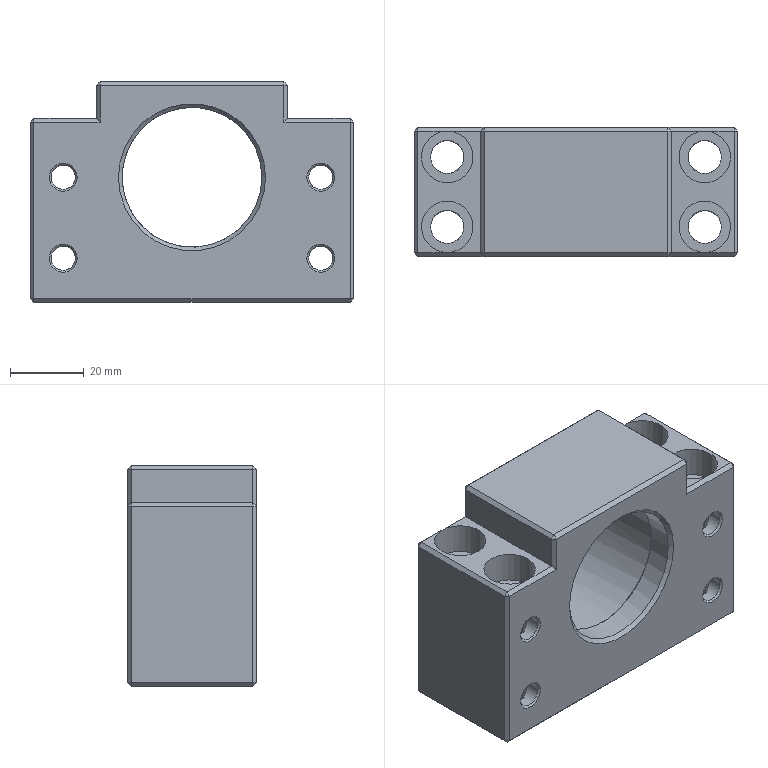Part | STEP file | BK-20_id1190_x_t | 1 solid | 90 faces | box 88 x 35 x 60 mm | volume 106061 mm3 | plane 49 | cylinder 26 | cone 15 | commonest cylinder face diameters 6.6 x12 4.2 x4 9 x4 14 x4 38 x1 42 x1